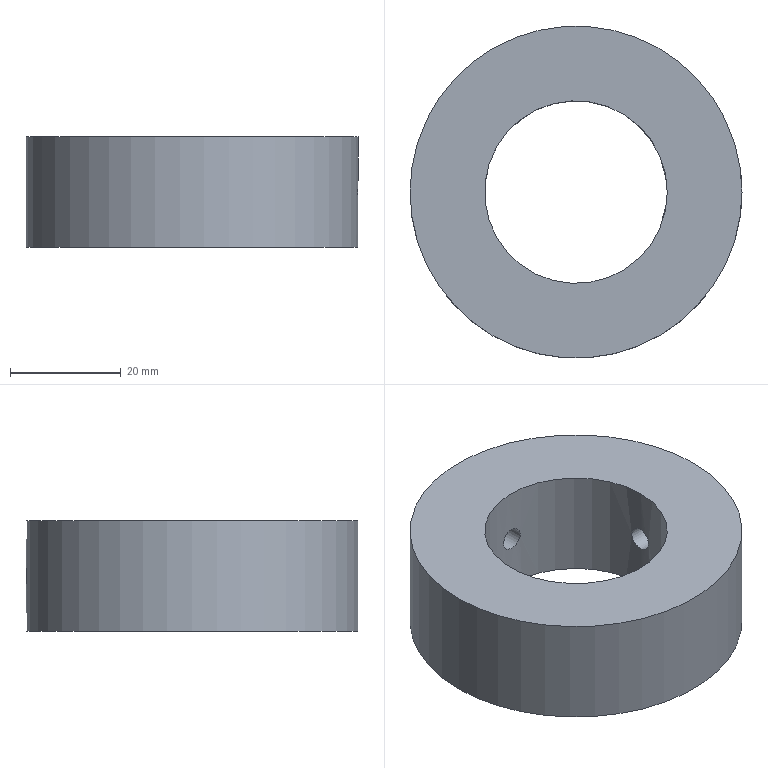Part | NX | 1 solid | 6 faces | box 60 x 60 x 20 mm | volume 39068 mm3 | cylinder 4 | plane 2 | commonest cylinder face diameters 4.2 x2 33 x1 60 x1
STEP:
#1=CARTESIAN_POINT('',(30.,0.,20.));
#2=VERTEX_POINT('',#1);
#3=CARTESIAN_POINT('',(0.,0.,20.));
#4=DIRECTION('',(0.,0.,1.));
#5=DIRECTION('',(1.,0.,0.));
#6=AXIS2_PLACEMENT_3D('',#3,#4,#5);
#7=CIRCLE('',#6,30.);
#8=EDGE_CURVE('',#2,#2,#7,.T.);
#9=ORIENTED_EDGE('',*,*,#8,.T.);
#10=EDGE_LOOP('',(#9));
#11=FACE_BOUND('',#10,.T.);
#12=CARTESIAN_POINT('',(16.5,0.,20.));
#13=VERTEX_POINT('',#12);
#14=CARTESIAN_POINT('',(0.,0.,20.));
#15=DIRECTION('',(0.,0.,1.));
#16=DIRECTION('',(1.,0.,0.));
#17=AXIS2_PLACEMENT_3D('',#14,#15,#16);
#18=CIRCLE('',#17,16.5);
#19=EDGE_CURVE('',#13,#13,#18,.T.);
#20=ORIENTED_EDGE('',*,*,#19,.F.);
#21=EDGE_LOOP('',(#20));
#22=FACE_BOUND('',#21,.T.);
#23=CARTESIAN_POINT('',(0.,0.,20.));
#24=DIRECTION('',(0.,0.,1.));
#25=DIRECTION('',(1.,0.,0.));
#26=AXIS2_PLACEMENT_3D('',#23,#24,#25);
#27=PLANE('',#26);
#28=ADVANCED_FACE('',(#11,#22),#27,.T.);
#29=CARTESIAN_POINT('',(30.,0.,0.));
#30=VERTEX_POINT('',#29);
#31=CARTESIAN_POINT('',(0.,0.,0.));
#32=DIRECTION('',(0.,0.,1.));
#33=DIRECTION('',(1.,0.,0.));
#34=AXIS2_PLACEMENT_3D('',#31,#32,#33);
#35=CIRCLE('',#34,30.);
#36=EDGE_CURVE('',#30,#30,#35,.T.);
#37=ORIENTED_EDGE('',*,*,#36,.F.);
#38=EDGE_LOOP('',(#37));
#39=FACE_BOUND('',#38,.T.);
#40=CARTESIAN_POINT('',(16.5,0.,0.));
#41=VERTEX_POINT('',#40);
#42=CARTESIAN_POINT('',(0.,0.,0.));
#43=DIRECTION('',(0.,0.,1.));
#44=DIRECTION('',(1.,0.,0.));
#45=AXIS2_PLACEMENT_3D('',#42,#43,#44);
#46=CIRCLE('',#45,16.5);
#47=EDGE_CURVE('',#41,#41,#46,.T.);
#48=ORIENTED_EDGE('',*,*,#47,.T.);
#49=EDGE_LOOP('',(#48));
#50=FACE_BOUND('',#49,.T.);
#51=CARTESIAN_POINT('',(0.,0.,0.));
#52=DIRECTION('',(0.,0.,1.));
#53=DIRECTION('',(1.,0.,0.));
#54=AXIS2_PLACEMENT_3D('',#51,#52,#53);
#55=PLANE('',#54);
#56=ADVANCED_FACE('',(#39,#50),#55,.F.);
#57=CARTESIAN_POINT('',(30.,0.,7.9));
#58=VERTEX_POINT('',#57);
#59=CARTESIAN_POINT('',(29.963,1.647,8.356));
#60=CARTESIAN_POINT('',(30.018,-0.0004179,7.672));
#61=CARTESIAN_POINT('',(29.963,-1.646,8.355));
#62=CARTESIAN_POINT('',(29.908,-2.327,9.998));
#63=CARTESIAN_POINT('',(29.963,-1.647,11.645));
#64=CARTESIAN_POINT('',(30.018,-0.0003537,12.327));
#65=CARTESIAN_POINT('',(29.963,1.644,11.647));
#66=CARTESIAN_POINT('',(29.908,2.327,10.002));
#67=CARTESIAN_POINT('',(29.963,1.647,8.356));
#68=CARTESIAN_POINT('',(30.018,-0.0004179,7.672));
#69=CARTESIAN_POINT('',(29.963,-1.646,8.355));
#70=B_SPLINE_CURVE_WITH_KNOTS('',3,(#59,#60,#61,#62,#63,#64,#65,#66,#67,#68,#69),.UNSPECIFIED.,.T.,.F.,(1,1,1,1,1,1,1,1,1,1,1,1,1,1,1),(-0.004925,-0.003283,-0.001642,0.,0.001642,0.003283,0.004925,0.006567,0.008209,0.00985,0.01149,0.01313,0.01478,0.01642,0.01806),.UNSPECIFIED.);
#71=EDGE_CURVE('',#58,#58,#70,.T.);
#72=ORIENTED_EDGE('',*,*,#71,.T.);
#73=EDGE_LOOP('',(#72));
#74=FACE_BOUND('',#73,.T.);
#75=CARTESIAN_POINT('',(0.,30.,12.1));
#76=VERTEX_POINT('',#75);
#77=CARTESIAN_POINT('',(1.647,29.963,11.644));
#78=CARTESIAN_POINT('',(-0.0004179,30.018,12.328));
#79=CARTESIAN_POINT('',(-1.646,29.963,11.645));
#80=CARTESIAN_POINT('',(-2.327,29.908,10.002));
#81=CARTESIAN_POINT('',(-1.647,29.963,8.355));
#82=CARTESIAN_POINT('',(-0.0003537,30.018,7.673));
#83=CARTESIAN_POINT('',(1.644,29.963,8.353));
#84=CARTESIAN_POINT('',(2.327,29.908,9.998));
#85=CARTESIAN_POINT('',(1.647,29.963,11.644));
#86=CARTESIAN_POINT('',(-0.0004179,30.018,12.328));
#87=CARTESIAN_POINT('',(-1.646,29.963,11.645));
#88=B_SPLINE_CURVE_WITH_KNOTS('',3,(#77,#78,#79,#80,#81,#82,#83,#84,#85,#86,#87),.UNSPECIFIED.,.T.,.F.,(1,1,1,1,1,1,1,1,1,1,1,1,1,1,1),(-0.004925,-0.003283,-0.001642,0.,0.001642,0.003283,0.004925,0.006567,0.008209,0.00985,0.01149,0.01313,0.01478,0.01642,0.01806),.UNSPECIFIED.);
#89=EDGE_CURVE('',#76,#76,#88,.T.);
#90=ORIENTED_EDGE('',*,*,#89,.T.);
#91=EDGE_LOOP('',(#90));
#92=FACE_BOUND('',#91,.T.);
#93=ORIENTED_EDGE('',*,*,#8,.F.);
#94=EDGE_LOOP('',(#93));
#95=FACE_BOUND('',#94,.T.);
#96=ORIENTED_EDGE('',*,*,#36,.T.);
#97=EDGE_LOOP('',(#96));
#98=FACE_BOUND('',#97,.T.);
#99=CARTESIAN_POINT('',(0.,0.,20.));
#100=DIRECTION('',(0.,0.,-1.));
#101=DIRECTION('',(-1.,0.,0.));
#102=AXIS2_PLACEMENT_3D('',#99,#100,#101);
#103=CYLINDRICAL_SURFACE('',#102,30.);
#104=ADVANCED_FACE('',(#74,#92,#95,#98),#103,.T.);
#105=CARTESIAN_POINT('',(16.5,0.,7.9));
#106=VERTEX_POINT('',#105);
#107=CARTESIAN_POINT('',(16.433,1.647,8.356));
#108=CARTESIAN_POINT('',(16.533,-0.0004054,7.672));
#109=CARTESIAN_POINT('',(16.433,-1.646,8.355));
#110=CARTESIAN_POINT('',(16.332,-2.327,9.998));
#111=CARTESIAN_POINT('',(16.433,-1.646,11.645));
#112=CARTESIAN_POINT('',(16.533,-0.0004828,12.327));
#113=CARTESIAN_POINT('',(16.433,1.644,11.647));
#114=CARTESIAN_POINT('',(16.332,2.327,10.002));
#115=CARTESIAN_POINT('',(16.433,1.647,8.356));
#116=CARTESIAN_POINT('',(16.533,-0.0004054,7.672));
#117=CARTESIAN_POINT('',(16.433,-1.646,8.355));
#118=B_SPLINE_CURVE_WITH_KNOTS('',3,(#107,#108,#109,#110,#111,#112,#113,#114,#115,#116,#117),.UNSPECIFIED.,.T.,.F.,(1,1,1,1,1,1,1,1,1,1,1,1,1,1,1),(-0.004929,-0.003286,-0.001643,0.,0.001643,0.003286,0.004929,0.006571,0.008214,0.009857,0.0115,0.01314,0.01479,0.01643,0.01807),.UNSPECIFIED.);
#119=EDGE_CURVE('',#106,#106,#118,.T.);
#120=ORIENTED_EDGE('',*,*,#119,.F.);
#121=EDGE_LOOP('',(#120));
#122=FACE_BOUND('',#121,.T.);
#123=CARTESIAN_POINT('',(0.,16.5,12.1));
#124=VERTEX_POINT('',#123);
#125=CARTESIAN_POINT('',(1.647,16.433,11.644));
#126=CARTESIAN_POINT('',(-0.0004054,16.533,12.328));
#127=CARTESIAN_POINT('',(-1.646,16.433,11.645));
#128=CARTESIAN_POINT('',(-2.327,16.332,10.002));
#129=CARTESIAN_POINT('',(-1.646,16.433,8.355));
#130=CARTESIAN_POINT('',(-0.0004828,16.533,7.673));
#131=CARTESIAN_POINT('',(1.644,16.433,8.353));
#132=CARTESIAN_POINT('',(2.327,16.332,9.998));
#133=CARTESIAN_POINT('',(1.647,16.433,11.644));
#134=CARTESIAN_POINT('',(-0.0004054,16.533,12.328));
#135=CARTESIAN_POINT('',(-1.646,16.433,11.645));
#136=B_SPLINE_CURVE_WITH_KNOTS('',3,(#125,#126,#127,#128,#129,#130,#131,#132,#133,#134,#135),.UNSPECIFIED.,.T.,.F.,(1,1,1,1,1,1,1,1,1,1,1,1,1,1,1),(-0.004929,-0.003286,-0.001643,0.,0.001643,0.003286,0.004929,0.006571,0.008214,0.009857,0.0115,0.01314,0.01479,0.01643,0.01807),.UNSPECIFIED.);
#137=EDGE_CURVE('',#124,#124,#136,.T.);
#138=ORIENTED_EDGE('',*,*,#137,.F.);
#139=EDGE_LOOP('',(#138));
#140=FACE_BOUND('',#139,.T.);
#141=ORIENTED_EDGE('',*,*,#19,.T.);
#142=EDGE_LOOP('',(#141));
#143=FACE_BOUND('',#142,.T.);
#144=ORIENTED_EDGE('',*,*,#47,.F.);
#145=EDGE_LOOP('',(#144));
#146=FACE_BOUND('',#145,.T.);
#147=CARTESIAN_POINT('',(0.,0.,20.));
#148=DIRECTION('',(0.,0.,-1.));
#149=DIRECTION('',(-1.,0.,0.));
#150=AXIS2_PLACEMENT_3D('',#147,#148,#149);
#151=CYLINDRICAL_SURFACE('',#150,16.5);
#152=ADVANCED_FACE('',(#122,#140,#143,#146),#151,.F.);
#153=ORIENTED_EDGE('',*,*,#137,.T.);
#154=EDGE_LOOP('',(#153));
#155=FACE_BOUND('',#154,.T.);
#156=ORIENTED_EDGE('',*,*,#89,.F.);
#157=EDGE_LOOP('',(#156));
#158=FACE_BOUND('',#157,.T.);
#159=CARTESIAN_POINT('',(0.,30.,10.));
#160=DIRECTION('',(0.,1.,0.));
#161=DIRECTION('',(0.,0.,1.));
#162=AXIS2_PLACEMENT_3D('',#159,#160,#161);
#163=CYLINDRICAL_SURFACE('',#162,2.1);
#164=ADVANCED_FACE('',(#155,#158),#163,.F.);
#165=ORIENTED_EDGE('',*,*,#119,.T.);
#166=EDGE_LOOP('',(#165));
#167=FACE_BOUND('',#166,.T.);
#168=ORIENTED_EDGE('',*,*,#71,.F.);
#169=EDGE_LOOP('',(#168));
#170=FACE_BOUND('',#169,.T.);
#171=CARTESIAN_POINT('',(30.,0.,10.));
#172=DIRECTION('',(1.,0.,0.));
#173=DIRECTION('',(0.,0.,-1.));
#174=AXIS2_PLACEMENT_3D('',#171,#172,#173);
#175=CYLINDRICAL_SURFACE('',#174,2.1);
#176=ADVANCED_FACE('',(#167,#170),#175,.F.);
#177=CLOSED_SHELL('',(#28,#56,#104,#152,#164,#176));
#178=MANIFOLD_SOLID_BREP('',#177);
#179=(LENGTH_UNIT()NAMED_UNIT(*)SI_UNIT(.MILLI.,.METRE.));
#180=UNCERTAINTY_MEASURE_WITH_UNIT(LENGTH_MEASURE(0.0508),#179,'','');
#181=(NAMED_UNIT(*)PLANE_ANGLE_UNIT()SI_UNIT($,.RADIAN.));
#182=(NAMED_UNIT(*)SI_UNIT($,.STERADIAN.)SOLID_ANGLE_UNIT());
#183=(GEOMETRIC_REPRESENTATION_CONTEXT(3)GLOBAL_UNCERTAINTY_ASSIGNED_CONTEXT((#180))GLOBAL_UNIT_ASSIGNED_CONTEXT((#179,#181,#182))REPRESENTATION_CONTEXT('',''));
#184=ADVANCED_BREP_SHAPE_REPRESENTATION('',(#178),#183);